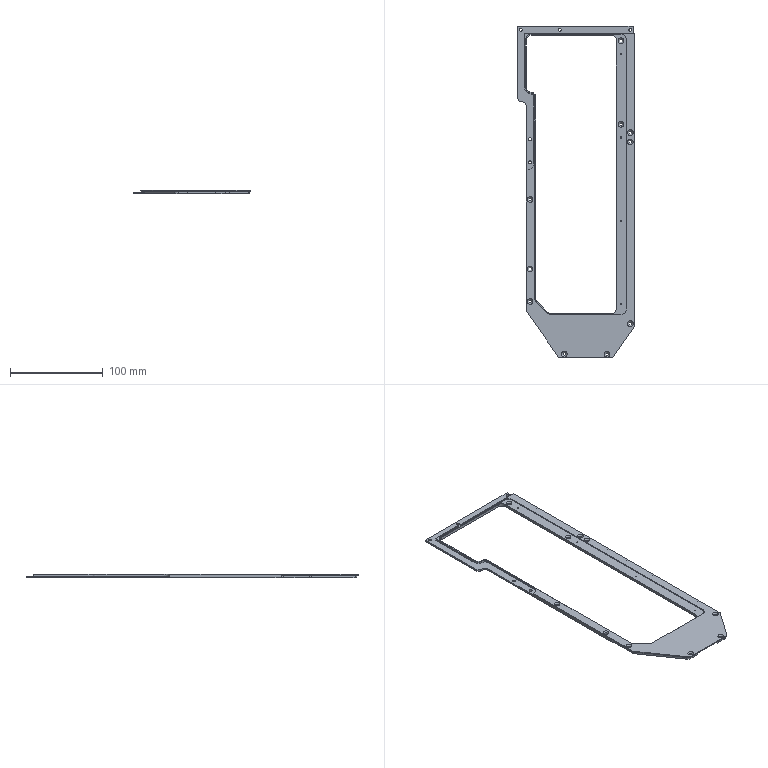NC program | NX | posted with a generic post | part box 127 x 358 x 4 mm
Whole program:
N10 G17 G21 G94 G90
(DRILLING , TOOL : CHAMFER_D8-90DEG)
N12 T01 M6
N14 G54
N16 G17 G0 G90 X64. Y-58.5 S2500 M3
N18 G43 Z20. H1
N20 G94 G81 G99 Z-2.3 F250. R3.
N22 X54.
N24 X-142.
N26 X-175. Y-33.5
N28 Y12.5
N30 X-118. Y49.5
N32 X-83.
N34 X-8.
N36 G80
N38 G0 X-8. Y49.5 Z20.
N40 M5
(PLANAR_MILL_2 , TOOL : D6-18-D6-50-3T-ROUGH)
N42 T03 M6
N44 G54
N46 G17 G0 G90 X31.2 Y59.5 S3500 M3
N48 G43 Z20. H3
N50 Z2.05
N52 G94 G1 Z-0.95 F1000.
N54 Y53.5
N56 G3 X32. Y52.7 R0.8
N58 G1 X98.935
N60 G2 X112.5 Y62.7 R14.2
N62 G1 X170.9
N64 G2 X178.2 Y55.4 R7.3
N66 G1 Y-63.5
N68 Y-69.5
N70 Z2.05
N72 G0 Z20.
N74 X27. Y59.5
N76 Z2.05
N78 G1 Z-0.95
N80 Y53.5
N82 G3 X32. Y48.5 R5.
N84 G1 X102.5
N86 G2 X112.5 Y58.5 R10.
N88 G1 X170.9
N90 G2 X174. Y55.4 R3.1
N92 G1 Y-63.5
N94 Y-69.5
N96 Z2.05
N98 G0 Z20.
N100 X31.2 Y59.5
N102 Z1.1
N104 G1 Z-1.9
N106 Y53.5
N108 G3 X32. Y52.7 R0.8
N110 G1 X98.935
N112 G2 X112.5 Y62.7 R14.2
N114 G1 X170.9
N116 G2 X178.2 Y55.4 R7.3
N118 G1 Y-63.5
N120 Y-69.5
N122 Z1.1
N124 G0 Z20.
N126 X27. Y59.5
N128 Z1.1
N130 G1 Z-1.9
N132 Y53.5
N134 G3 X32. Y48.5 R5.
N136 G1 X102.5
N138 G2 X112.5 Y58.5 R10.
N140 G1 X170.9
N142 G2 X174. Y55.4 R3.1
N144 G1 Y-63.5
N146 Y-69.5
N148 Z1.1
N150 G0 Z20.
(PLANAR_MILL_2_COPY , TOOL : D6-18-D6-50-3T-ROUGH)
N152 X90.5 Y57.5
N154 Z0.1
N156 G1 Z-1.9
N158 Y54.5
N160 G3 X92.5 Y52.5 R2.
N162 X98.5 Y58.5 R6.
N164 G2 X102.5 Y62.5 R4.
N166 G1 X175.
N168 G2 X178. Y59.5 R3.
N170 G1 Y53.5
N172 G3 X180. Y51.5 R2.
N174 G1 X183.
N176 Z0.1
N178 G0 Z20.
(PLANAR_MILL_3 , TOOL : D6-18-D6-50-3T-ROUGH)
N180 X19. Y-48.4
N182 Z2.1
N184 G1 Z-0.9
N186 Y-51.4
N188 X164.
N190 G3 X166.9 Y-48.5 R2.9
N192 G1 Y48.5
N194 G3 X164. Y51.4 R2.9
N196 G1 X112.5
N198 G3 X109.6 Y48.5 R2.9
N200 G2 X102.5 Y41.4 R7.1
N202 G1 X-114.787
N204 G3 X-116.837 Y40.551 R2.9
N206 G1 X-128.051 Y29.337
N208 G3 X-128.9 Y27.287 R2.9
N210 G1 Y-48.5
N212 G3 X-126. Y-51.4 R2.9
N214 G1 X19.
N216 Y-48.4
N218 Z2.1
N220 G0 Z20.
(PLANAR_MILL_3_COPY , TOOL : D6-18-D6-50-3T-ROUGH)
N222 X-123.5 Y-32.5
N224 Z2.1
N226 G1 Z-0.9
N228 Y-38.5
N230 Y-46.
N232 X161.5
N234 Y-38.5
N236 Y-32.5
N238 Z2.1
N240 G0 Z20.
N242 M5
(PLANAR_MILL_2_COPY_1 , TOOL : D6-18-D6-50-3T-FINISH)
N244 T04 M6
N246 G54
N248 G17 G0 G90 X31.135 Y59.697 S3500 M3
N250 G43 Z20. H4
N252 Z2.
N254 G94 G1 Z-1. F800.
N256 G41 X31.1 Y59.5 D4
N258 Y53.5
N260 G3 X32. Y52.6 R0.9
N262 G1 X99.009
N264 G2 X112.5 Y62.6 R14.1
N266 G1 X170.9
N268 G2 X178.1 Y55.4 R7.2
N270 G1 Y-63.5
N272 Y-69.5
N274 G40
N276 X178.135 Y-69.697
N278 Z2.
N280 G0 Z20.
N282 X26.935 Y59.697
N284 Z2.
N286 G1 Z-1.
N288 G41 X26.9 Y59.5
N290 Y53.5
N292 G3 X32. Y48.4 R5.1
N294 G1 X102.5
N296 X102.565 Y48.387
N298 X102.613 Y48.435
N300 X102.6 Y48.5
N302 G2 X112.5 Y58.4 R9.9
N304 G1 X170.9
N306 G2 X173.9 Y55.4 R3.
N308 G1 Y-63.5
N310 Y-69.5
N312 G40
N314 X173.935 Y-69.697
N316 Z2.
N318 G0 Z20.
N320 X31.135 Y59.697
N322 Z1.
N324 G1 Z-2.
N326 G41 X31.1 Y59.5
N328 Y53.5
N330 G3 X32. Y52.6 R0.9
N332 G1 X99.009
N334 G2 X112.5 Y62.6 R14.1
N336 G1 X170.9
N338 G2 X178.1 Y55.4 R7.2
N340 G1 Y-63.5
N342 Y-69.5
N344 G40
N346 X178.135 Y-69.697
N348 Z1.
N350 G0 Z20.
N352 X26.935 Y59.697
N354 Z1.
N356 G1 Z-2.
N358 G41 X26.9 Y59.5
N360 Y53.5
N362 G3 X32. Y48.4 R5.1
N364 G1 X102.5
N366 X102.565 Y48.387
N368 X102.613 Y48.435
N370 X102.6 Y48.5
N372 G2 X112.5 Y58.4 R9.9
N374 G1 X170.9
N376 G2 X173.9 Y55.4 R3.
N378 G1 Y-63.5
N380 Y-69.5
N382 G40
N384 X173.935 Y-69.697
N386 Z1.
N388 G0 Z20.
(PLANAR_MILL_2_COPY_COPY , TOOL : D6-18-D6-50-3T-FINISH)
N390 X90.5 Y59.5
N392 Z0.
N394 G1 Z-2.
N396 Y53.5
N398 G3 X92.5 Y51.5 R2.
N400 X99.5 Y58.5 R7.
N402 G2 X102.5 Y61.5 R3.
N404 G1 X174.
N406 G2 X177. Y58.5 R3.
N408 G1 Y53.5
N410 G3 X179. Y51.5 R2.
N412 G1 X185.
N414 Z0.
N416 G0 Z20.
(PLANAR_MILL_3_COPY_1_COPY , TOOL : D6-18-D6-50-3T-FINISH)
N418 X-113.787 Y37.5
N420 Z2.
N422 G1 Z-1.
N424 G41 X-116.201 Y39.914
N426 X-127.414 Y28.701
N428 G3 X-128. Y27.287 R2.
N430 G1 Y-48.5
N432 G3 X-126. Y-50.5 R2.
N434 G1 X164.
N436 G3 X166. Y-48.5 R2.
N438 G1 Y48.5
N440 G3 X164. Y50.5 R2.
N442 G1 X112.5
N444 G3 X110.5 Y48.5 R2.
N446 G2 X102.5 Y40.5 R8.
N448 G1 X-114.787
N450 G3 X-116.201 Y39.914 R2.
N452 G40
N454 G1 X-113.787 Y37.5
N456 Z2.
N458 G0 Z20.
(PLANAR_MILL_3_COPY_1 , TOOL : D6-18-D6-50-3T-FINISH)
N460 X-114.787 Y38.5
N462 Z2.
N464 G1 Z-1.
N466 G41 X-116.908 Y40.621
N468 X-128.121 Y29.408
N470 G3 X-129. Y27.287 R3.
N472 G1 Y-48.5
N474 G3 X-126. Y-51.5 R3.
N476 G1 X164.
N478 G3 X167. Y-48.5 R3.
N480 G1 Y48.5
N482 G3 X164. Y51.5 R3.
N484 G1 X112.5
N486 G3 X109.5 Y48.5 R3.
N488 G2 X102.5 Y41.5 R7.
N490 G1 X-114.787
N492 G3 X-116.908 Y40.621 R3.
N494 G40
N496 G1 X-114.787 Y38.5
N498 Z2.
N500 G0 Z20.
(PLANAR_MILL_3_COPY_COPY , TOOL : D6-18-D6-50-3T-FINISH)
N502 X-123.465 Y-32.303
N504 Z2.
N506 G1 Z-1.
N508 G41 X-123.5 Y-32.5
N510 Y-38.5
N512 Y-46.
N514 X161.5
N516 Y-38.5
N518 Y-32.5
N520 G40
N522 X161.465 Y-32.303
N524 Z2.
N526 G0 Z20.
N528 M5
(DRILLING_2 , TOOL : CHAMFER_D8-90DEG)
N530 T01 M6
N532 G54
N534 G17 G0 G90 X163. Y-48.5 S2500 M3
N536 G43 Z20. H1
N538 G94 G81 G99 Z-3.3 F200. R2.
N540 X73.
N542 G80
N544 G0 X73. Y-48.5 Z20.
(DRILLING_1 , TOOL : CHAMFER_D8-90DEG)
N546 X149.
N548 G81 Z-1.8 F200. R2.
N550 X59.
N552 X-31.
N554 X-121.
N556 G80
N558 G0 X-121. Y-48.5 Z20.
N560 M5
(DRILLING_3 , TOOL : DRILL_D1.84-11-D3-40)
N562 T20 M6
N564 G54
N566 G17 G0 G90 X149. Y-48.5 S1600 M3
N568 G43 Z20. H20
N570 G94 G83 G99 Z-6. F100. Q1. R2.
N572 X59.
N574 X-31.
N576 X-121.
N578 G80
N580 G0 X-121. Y-48.5 Z20.
N582 M5
(PLANAR_MILL_5 , TOOL : CHAMFER_D3-90DEG)
N584 T08 M6
N586 G54
N588 G17 G0 G90 X173.597 Y-62.535 S3000 M3
N590 G43 Z20. H8
N592 Z1.
N594 G94 G1 Z-1. F1000.
N596 G41 X173.4 Y-62.5 D8
N598 G3 X172.4 Y-63.5 R1.
N600 G2 X170.9 Y-65. R1.5
N602 G1 X-143.369
N604 G2 X-145.377 Y-64.367 R3.5
N606 G1 X-179.008 Y-40.819
N608 G2 X-180.5 Y-37.952 R3.5
N610 G1 Y17.098
N612 G2 X-179.008 Y19.965 R3.5
N614 G1 X-129.877 Y54.367
N616 G2 X-127.869 Y55. R3.5
N618 G1 X23.9
N620 G2 X25.4 Y53.5 R1.5
N622 G3 X32. Y46.9 R6.6
N624 G1 X102.5
N626 G3 X104.1 Y48.5 R1.6
N628 G2 X112.5 Y56.9 R8.4
N630 G1 X170.9
N632 G2 X172.4 Y55.4 R1.5
N634 G1 Y-63.5
N636 G3 X173.4 Y-64.5 R1.
N638 G40
N640 G1 X173.597 Y-64.465
N642 Z1.
N644 G0 Z20.
(PLANAR_MILL_6 , TOOL : CHAMFER_D3-90DEG)
N646 X24.935 Y56.297
N648 Z-0.6
N650 G1 Z-2.6
N652 G41 X24.9 Y56.1
N654 G3 X26.9 Y54.1 R2.
N656 G1 X92.5
N658 G3 X96.9 Y58.5 R4.4
N660 G2 X102.5 Y64.1 R5.6
N662 G1 X179.
N664 G2 X179.6 Y63.5 R0.6
N666 G1 Y-61.5
N668 G3 X181.6 Y-63.5 R2.
N670 G40
N672 G1 X181.797 Y-63.465
N674 Z-0.6
N676 G0 Z20.
(PLANAR_MILL_5_COPY , TOOL : CHAMFER_D3-90DEG)
N678 X164.965 Y52.588
N680 Z1.4
N682 G1 Z-0.6
N684 G41 X165. Y52.785
N686 Y52.9
N688 G3 X164. Y53.9 R1.
N690 G1 X112.5
N692 G3 X107.1 Y48.5 R5.4
N694 G2 X102.5 Y43.9 R4.6
N696 G1 X-114.787
N698 G3 X-118.605 Y42.318 R5.4
N700 G1 X-129.818 Y31.105
N702 G3 X-131.4 Y27.287 R5.4
N704 G1 Y-48.5
N706 G3 X-126. Y-53.9 R5.4
N708 G1 X164.
N710 G3 X169.4 Y-48.5 R5.4
N712 G1 Y48.5
N714 G3 X164. Y53.9 R5.4
N716 X163. Y52.9 R1.
N718 G40
N720 G1 X163.035 Y52.703
N722 Z1.4
N724 G0 Z20.
N726 M5
(DRILLING_3_COPY , TOOL : FORMTAP_M2-12-D3-39)
N728 T21 M6
N730 G54
N732 G17 G0 G90 X149. Y-48.5 S300 M3
N734 G43 Z20. H21
N736 G84 G94 G99 Z-5.5 F120. R2.
N738 X59.
N740 X-31.
N742 X-121.
N744 G80
N746 G0 X-121. Y-48.5 Z20.
N748 M5
(PLANAR_MILL_4 , TOOL : D6-18-D6-50-3T-ROUGH)
N750 T03 M6
N752 G54
N754 G17 G0 G90 X110.726 Y49.025 S3500 M3
N756 G43 Z20. H3
N758 Z-0.5
N760 G94 G1 X110.65 Y48.835 F1500.
N762 Y48.5
N764 Y47.8 Z-0.501
N766 X110.268 Y45.935 Z-0.502
N768 X109.464 Y44.209 Z-0.503
N770 X108.284 Y42.716 Z-0.504
N772 X106.791 Y41.536 Z-0.505
N774 X105.065 Y40.732 Z-0.506
N776 X103.2 Y40.35 Z-0.507
N778 X-115.121 Z-0.621
N780 X-115.858 Y40.045
N782 X-127.545 Y28.358 Z-0.63
N784 X-127.85 Y27.621
N786 Y-38.835 Z-0.665
N788 X-127.569 Y-39.535 Z-0.666
N790 X-127.035 Y-40.069
N792 X-126.335 Y-40.35
N794 X164.335 Z-0.819
N796 X165.035 Y-40.069
N798 X165.569 Y-39.535
N800 X165.85 Y-38.835 Z-0.82
N802 Y48.835 Z-0.866
N804 X165.569 Y49.535
N806 X165.035 Y50.069
N808 X164.335 Y50.35 Z-0.867
N810 X112.165 Z-0.894
N812 X111.465 Y50.069 Z-0.895
N814 X110.931 Y49.535
N816 X110.65 Y48.835
N818 Y48.5 Z-0.896
N820 Y47.8
N822 X110.268 Y45.935 Z-0.897
N824 X109.464 Y44.209 Z-0.898
N826 X108.284 Y42.716 Z-0.899
N828 X106.791 Y41.536 Z-0.9
N830 X105.065 Y40.732 Z-0.901
N832 X103.2 Y40.35 Z-0.902
N834 X-115.121 Z-1.016
N836 X-115.858 Y40.045 Z-1.017
N838 X-127.545 Y28.358 Z-1.025
N840 X-127.85 Y27.621 Z-1.026
N842 Y-38.835 Z-1.061
N844 X-127.569 Y-39.535
N846 X-127.035 Y-40.069
N848 X-126.335 Y-40.35 Z-1.062
N850 X164.335 Z-1.214
N852 X165.035 Y-40.069
N854 X165.569 Y-39.535 Z-1.215
N856 X165.85 Y-38.835
N858 Y48.835 Z-1.261
N860 X165.569 Y49.535
N862 X165.035 Y50.069 Z-1.262
N864 X164.335 Y50.35
N866 X112.165 Z-1.289
N868 X111.465 Y50.069 Z-1.29
N870 X110.931 Y49.535
N872 X110.65 Y48.835 Z-1.291
N874 Y48.5
N876 Y47.8
N878 X110.268 Y45.935 Z-1.292
N880 X109.464 Y44.209 Z-1.293
N882 X108.284 Y42.716 Z-1.294
N884 X106.791 Y41.536 Z-1.295
N886 X105.065 Y40.732 Z-1.296
N888 X103.2 Y40.35 Z-1.297
N890 X-115.121 Z-1.411
N892 X-115.858 Y40.045 Z-1.412
N894 X-127.545 Y28.358 Z-1.421
N896 X-127.85 Y27.621
N898 Y-38.835 Z-1.456
N900 X-127.569 Y-39.535
N902 X-127.035 Y-40.069 Z-1.457
N904 X-126.335 Y-40.35
N906 X164.335 Z-1.609
N908 X165.035 Y-40.069 Z-1.61
N910 X165.569 Y-39.535
N912 X165.85 Y-38.835
N914 Y48.835 Z-1.656
N916 X165.569 Y49.535 Z-1.657
N918 X165.035 Y50.069
N920 X164.335 Y50.35
N922 X112.165 Z-1.685
N924 X111.465 Y50.069
N926 X110.931 Y49.535 Z-1.686
N928 X110.65 Y48.835
N930 Y48.5
N932 Y47.8
N934 X110.268 Y45.935 Z-1.687
N936 X109.464 Y44.209 Z-1.688
N938 X108.284 Y42.716 Z-1.689
N940 X106.791 Y41.536 Z-1.69
N942 X105.065 Y40.732 Z-1.691
N944 X103.2 Y40.35 Z-1.692
N946 X-115.121 Z-1.807
N948 X-115.858 Y40.045
N950 X-127.545 Y28.358 Z-1.816
N952 X-127.85 Y27.621
N954 Y-38.835 Z-1.851
N956 X-127.569 Y-39.535
N958 X-127.035 Y-40.069 Z-1.852
N960 X-126.335 Y-40.35
N962 X164.335 Z-2.004
N964 X165.035 Y-40.069 Z-2.005
N966 X165.569 Y-39.535
N968 X165.85 Y-38.835 Z-2.006
N970 Y48.835 Z-2.052
N972 X165.569 Y49.535
N974 X165.035 Y50.069
N976 X164.335 Y50.35 Z-2.053
N978 X112.165 Z-2.08
N980 X111.465 Y50.069
N982 X110.931 Y49.535 Z-2.081
N984 X110.65 Y48.835
N986 Y48.5
N988 Y47.8 Z-2.082
N990 X110.268 Y45.935 Z-2.083
N992 X109.464 Y44.209 Z-2.084
N994 X108.284 Y42.716 Z-2.085
N996 X106.791 Y41.536 Z-2.086
N998 X105.065 Y40.732 Z-2.087
N1000 X103.2 Y40.35 Z-2.088
N1002 X-115.121 Z-2.202
N1004 X-115.858 Y40.045
N1006 X-127.545 Y28.358 Z-2.211
N1008 X-127.85 Y27.621 Z-2.212
N1010 Y-38.835 Z-2.246
N1012 X-127.569 Y-39.535 Z-2.247
N1014 X-127.035 Y-40.069
N1016 X-126.335 Y-40.35 Z-2.248
N1018 X164.335 Z-2.4
N1020 X165.035 Y-40.069
N1022 X165.569 Y-39.535 Z-2.401
N1024 X165.85 Y-38.835
N1026 Y48.835 Z-2.447
N1028 X165.569 Y49.535
N1030 X165.035 Y50.069 Z-2.448
N1032 X164.335 Y50.35
N1034 X112.165 Z-2.475
N1036 X111.465 Y50.069 Z-2.476
N1038 X110.931 Y49.535
N1040 X110.65 Y48.835
N1042 Y48.5 Z-2.477
N1044 Y47.8
N1046 X110.268 Y45.935 Z-2.478
N1048 X109.464 Y44.209 Z-2.479
N1050 X108.284 Y42.716 Z-2.48
N1052 X106.791 Y41.536 Z-2.481
N1054 X105.065 Y40.732 Z-2.482
N1056 X103.2 Y40.35 Z-2.483
N1058 X-115.121 Z-2.597
N1060 X-115.858 Y40.045 Z-2.598
N1062 X-127.545 Y28.358 Z-2.606
N1064 X-127.85 Y27.621 Z-2.607
N1066 Y-38.835 Z-2.642
N1068 X-127.569 Y-39.535
N1070 X-127.035 Y-40.069
N1072 X-126.335 Y-40.35 Z-2.643
N1074 X164.335 Z-2.795
N1076 X165.035 Y-40.069
N1078 X165.569 Y-39.535 Z-2.796
N1080 X165.85 Y-38.835
N1082 Y48.835 Z-2.842
N1084 X165.569 Y49.535
N1086 X165.035 Y50.069 Z-2.843
N1088 X164.335 Y50.35
N1090 X112.165 Z-2.871
N1092 X111.465 Y50.069
N1094 X110.931 Y49.535
N1096 X110.65 Y48.835 Z-2.872
N1098 Y48.5
N1100 Y47.8
N1102 X110.268 Y45.935 Z-2.873
N1104 X109.464 Y44.209 Z-2.874
N1106 X108.284 Y42.716 Z-2.875
N1108 X106.791 Y41.536 Z-2.876
N1110 X105.065 Y40.732 Z-2.877
N1112 X103.2 Y40.35 Z-2.878
N1114 X-115.121 Z-2.993
N1116 X-115.858 Y40.045
N1118 X-127.545 Y28.358 Z-3.002
N1120 X-127.85 Y27.621
N1122 Y-38.835 Z-3.037
N1124 X-127.569 Y-39.535
N1126 X-127.035 Y-40.069 Z-3.038
N1128 X-126.335 Y-40.35
N1130 X164.335 Z-3.19
N1132 X165.035 Y-40.069 Z-3.191
N1134 X165.569 Y-39.535
N1136 X165.85 Y-38.835
N1138 Y48.835 Z-3.237
N1140 X165.569 Y49.535 Z-3.238
N1142 X165.035 Y50.069
N1144 X164.335 Y50.35 Z-3.239
N1146 X112.165 Z-3.266
N1148 X111.465 Y50.069
N1150 X110.931 Y49.535 Z-3.267
N1152 X110.65 Y48.835
N1154 Y48.5
N1156 Y47.8 Z-3.268
N1158 X110.268 Y45.935 Z-3.269
N1160 X109.464 Y44.209 Z-3.27
N1162 X108.284 Y42.716 Z-3.271
N1164 X106.791 Y41.536 Z-3.272
N1166 X105.065 Y40.732 Z-3.273
N1168 X103.2 Y40.35 Z-3.274
N1170 X-115.121 Z-3.388
N1172 X-115.858 Y40.045
N1174 X-127.545 Y28.358 Z-3.397
N1176 X-127.85 Y27.621
N1178 Y-38.835 Z-3.432
N1180 X-127.569 Y-39.535 Z-3.433
N1182 X-127.035 Y-40.069
N1184 X-126.335 Y-40.35
N1186 X164.335 Z-3.586
N1188 X165.035 Y-40.069
N1190 X165.569 Y-39.535
N1192 X165.85 Y-38.835 Z-3.587
N1194 Y48.835 Z-3.633
N1196 X165.569 Y49.535
N1198 X165.035 Y50.069
N1200 X164.335 Y50.35 Z-3.634
N1202 X112.165 Z-3.661
N1204 X111.465 Y50.069 Z-3.662
N1206 X110.931 Y49.535
N1208 X110.65 Y48.835
N1210 Y48.5
N1212 Y47.8 Z-3.663
N1214 X110.268 Y45.935 Z-3.664
N1216 X109.464 Y44.209 Z-3.665
N1218 X108.284 Y42.716 Z-3.666
N1220 X106.791 Y41.536 Z-3.667
N1222 X105.065 Y40.732 Z-3.668
N1224 X103.2 Y40.35 Z-3.669
N1226 X-115.121 Z-3.783
N1228 X-115.858 Y40.045 Z-3.784
N1230 X-127.545 Y28.358 Z-3.792
N1232 X-127.85 Y27.621 Z-3.793
N1234 Y-38.835 Z-3.827
N1236 X-127.569 Y-39.535 Z-3.828
N1238 X-127.035 Y-40.069
N1240 X-126.335 Y-40.35 Z-3.829
N1242 X164.335 Z-3.981
N1244 X165.035 Y-40.069
N1246 X165.569 Y-39.535 Z-3.982
N1248 X165.85 Y-38.835
N1250 Y48.835 Z-4.028
N1252 X165.569 Y49.535
N1254 X165.035 Y50.069 Z-4.029
N1256 X164.335 Y50.35
N1258 X112.165 Z-4.056
N1260 X111.465 Y50.069 Z-4.057
N1262 X110.931 Y49.535
N1264 X110.65 Y48.835 Z-4.058
N1266 Y48.5
N1268 Y47.8
N1270 X110.268 Y45.935 Z-4.059
N1272 X109.464 Y44.209 Z-4.06
N1274 X108.284 Y42.716 Z-4.061
N1276 X106.791 Y41.536 Z-4.062
N1278 X105.065 Y40.732 Z-4.063
N1280 X103.2 Y40.35 Z-4.064
N1282 X-115.121 Z-4.178
N1284 X-115.858 Y40.045 Z-4.179
N1286 X-127.545 Y28.358 Z-4.188
N1288 X-127.85 Y27.621
N1290 Y-38.835 Z-4.223
N1292 X-127.569 Y-39.535
N1294 X-127.035 Y-40.069 Z-4.224
N1296 X-126.335 Y-40.35
N1298 X-126.
N1300 X19. Z-4.3
N1302 X164.
N1304 G3 X165.85 Y-38.5 R1.85
N1306 G1 Y48.5
N1308 G3 X164. Y50.35 R1.85
N1310 G1 X112.5
N1312 G3 X110.65 Y48.5 R1.85
N1314 G2 X102.5 Y40.35 R8.15
N1316 G1 X-114.787
N1318 G3 X-116.095 Y39.808 R1.85
N1320 G1 X-127.308 Y28.595
N1322 G3 X-127.85 Y27.287 R1.85
N1324 G1 Y-38.5
N1326 G3 X-126. Y-40.35 R1.85
N1328 G1 X19.
N1330 Z-3.8
N1332 G0 Z20.
N1334 M5
(PLANAR_MILL_4_COPY , TOOL : D6-18-D6-50-3T-FINISH)
N1336 T04 M6
N1338 G54
N1340 G17 G0 G90 X-126.217 Y28.252 S3500 M3
N1342 G43 Z20. H4
N1344 Z-2.3
N1346 G94 G1 Z-4.3 F800.
N1348 G41 X-126.414 Y28.287 D4
N1350 X-127.
N1352 G3 X-128. Y27.287 R1.
N1354 G1 Y-38.5
N1356 G3 X-126. Y-40.5 R2.
N1358 G1 X164.
N1360 G3 X166. Y-38.5 R2.
N1362 G1 Y48.5
N1364 G3 X164. Y50.5 R2.
N1366 G1 X112.5
N1368 G3 X110.5 Y48.5 R2.
N1370 G2 X102.5 Y40.5 R8.
N1372 G1 X-114.787
N1374 G3 X-116.201 Y39.914 R2.
N1376 G1 X-127.414 Y28.701
N1378 G3 X-128. Y27.287 R2.
N1380 X-127. Y26.287 R1.
N1382 G40
N1384 G1 X-126.803 Y26.322
N1386 Y28.252
N1388 G41 X-127. Y28.287
N1390 G3 X-128. Y27.287 R1.
N1392 G1 Y-38.5
N1394 G3 X-126. Y-40.5 R2.
N1396 G1 X164.
N1398 G3 X166. Y-38.5 R2.
N1400 G1 Y48.5
N1402 G3 X164. Y50.5 R2.
N1404 G1 X112.5
N1406 G3 X110.5 Y48.5 R2.
N1408 G2 X102.5 Y40.5 R8.
N1410 G1 X-114.787
N1412 G3 X-116.201 Y39.914 R2.
N1414 G1 X-127.414 Y28.701
N1416 G3 X-128. Y27.287 R2.
N1418 X-127. Y26.287 R1.
N1420 G40
N1422 G1 X-126.803 Y26.322
N1424 Z-2.3
N1426 G0 Z20.
N1428 M5
(PLANAR_MILL_5_COPY_COPY , TOOL : CHAMFER_D3-90DEG)
N1430 T08 M6
N1432 G54
N1434 G17 G0 G90 X-127.697 Y30.398 S3000 M3
N1436 G43 Z20. H8
N1438 Z0.4
N1440 G94 G1 Z-1.6 F1000.
N1442 G3 X-129.111 Y30.398 R1.
N1444 X-130.4 Y27.287 R4.4
N1446 G1 Y-38.5
N1448 G3 X-126. Y-42.9 R4.4
N1450 G1 X164.
N1452 G3 X168.4 Y-38.5 R4.4
N1454 G1 Y48.5
N1456 G3 X164. Y52.9 R4.4
N1458 G1 X112.5
N1460 G3 X108.1 Y48.5 R4.4
N1462 G2 X102.5 Y42.9 R5.6
N1464 G1 X-114.787
N1466 G3 X-117.898 Y41.611 R4.4
N1468 G1 X-129.111 Y30.398
N1470 G3 X-129.111 Y28.984 R1.
N1472 G1 X-129.005 Y28.878
N1474 Z0.4
N1476 G0 Z20.
N1478 M5
N1480 M2